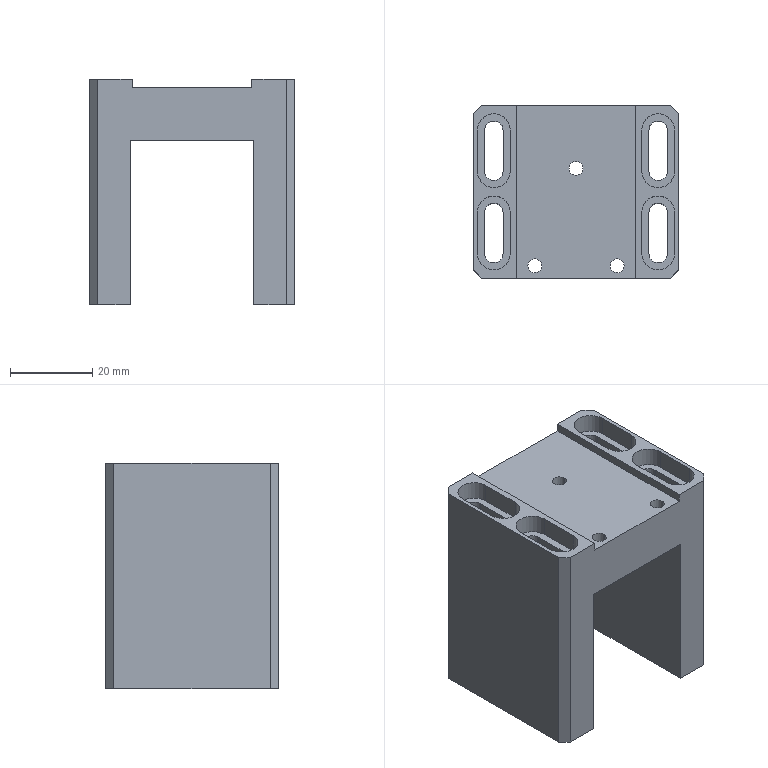Part | SolidWorks | features HoleWzd 2, ICE 2, Chamfer 1, Extrusion 1 | 1 solid | 60 faces | box 50 x 42 x 55 mm | volume 47186 mm3 | plane 38 | cylinder 22 | commonest cylinder face diameters 4.5 x8 8 x8 3.4 x6